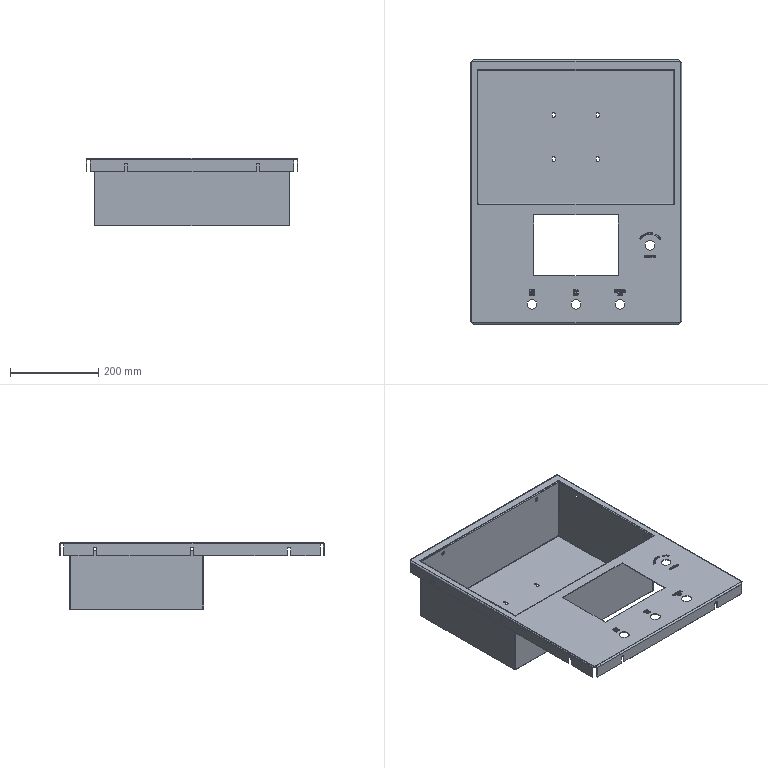Part | SolidWorks | features ICE 7, EdgeFlange 3, Cut 1, FlatPattern 1, SMBaseFlange 1, SheetMetal 1 | 1 solid | 1433 faces | box 480 x 600 x 153 mm | volume 803618 mm3 | plane 966 | spline 407 | cylinder 60 | commonest cylinder face diameters 8 x26 6 x8 22.5 x8 2 x5 5 x5 4 x4